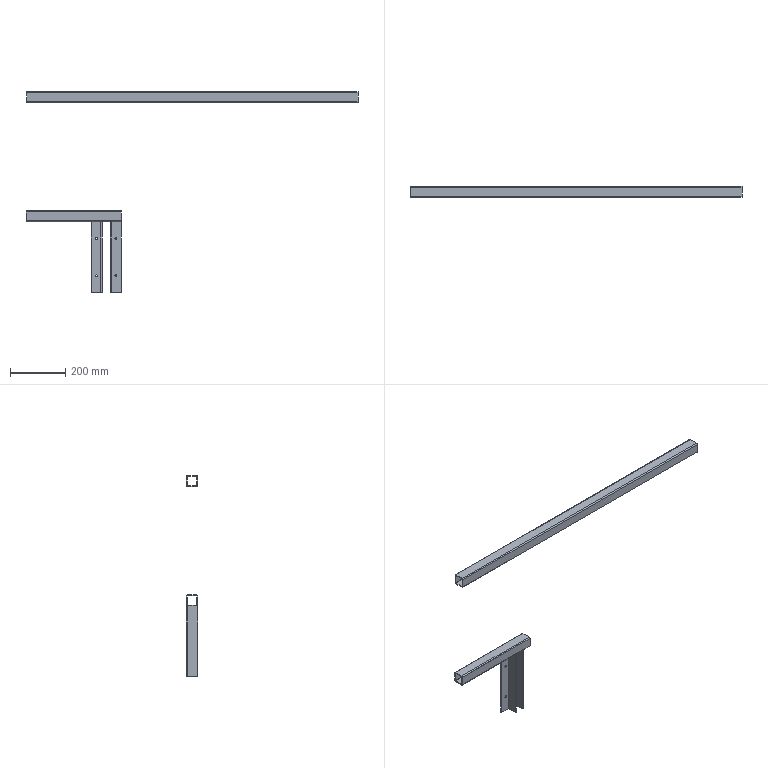Part | 4 solids | 60 faces | box 1200 x 40 x 726 mm | volume 855748 mm3 | plane 36 | cylinder 24 | commonest cylinder face diameters 2 x8 6.8 x8 8 x8